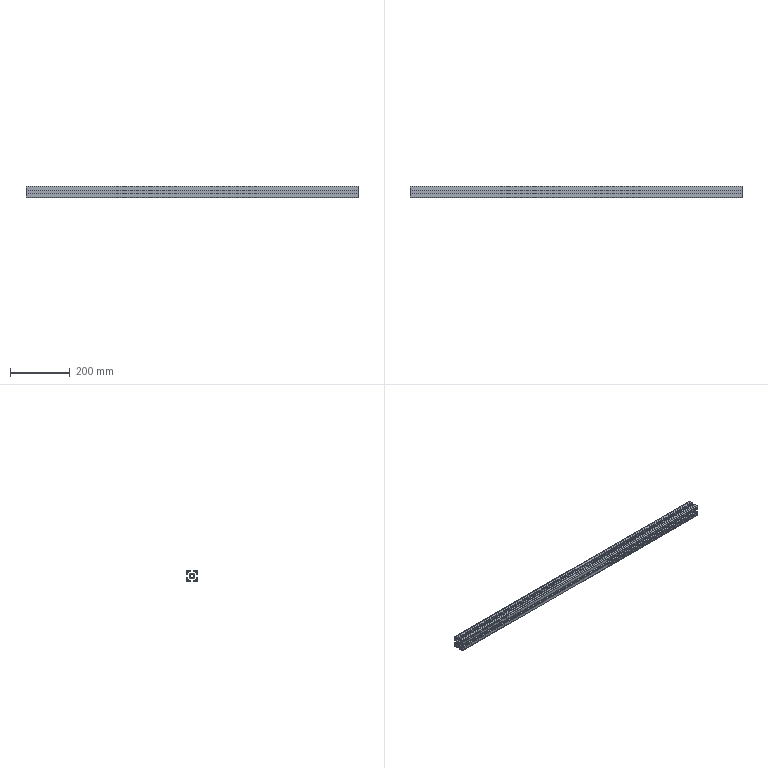Part | STEP file | AL PROFILE 4040 L 1110 | 1 solid | 137 faces | box 1110 x 40 x 40 mm | volume 616920 mm3 | plane 110 | cylinder 27 | commonest cylinder face diameters 3 x10 5.5 x8 10 x5 6 x4